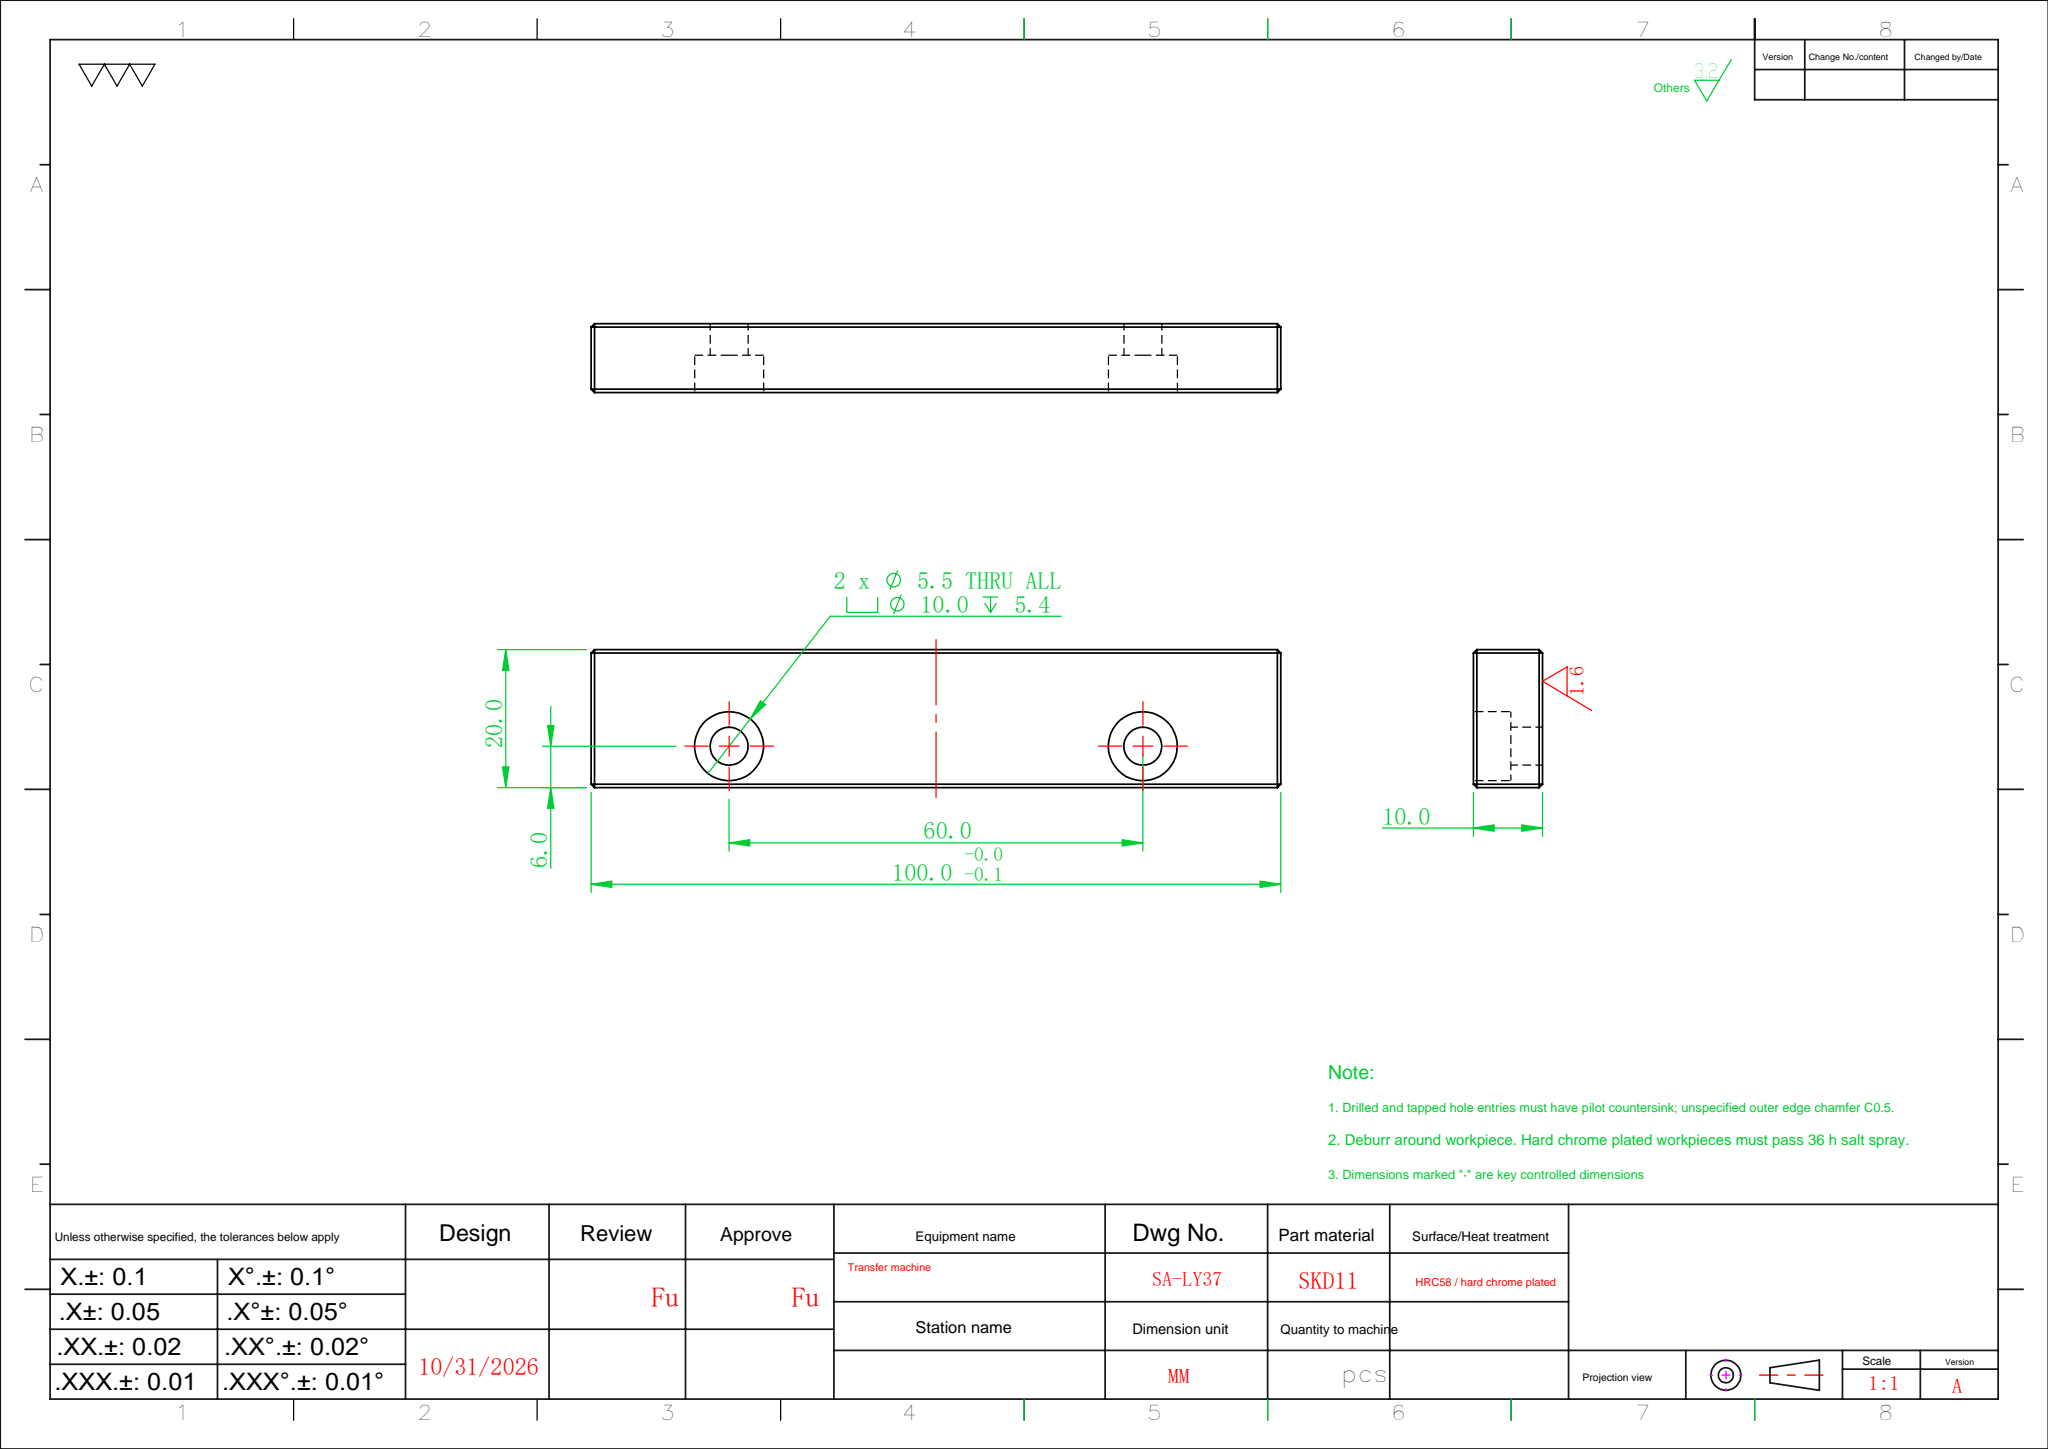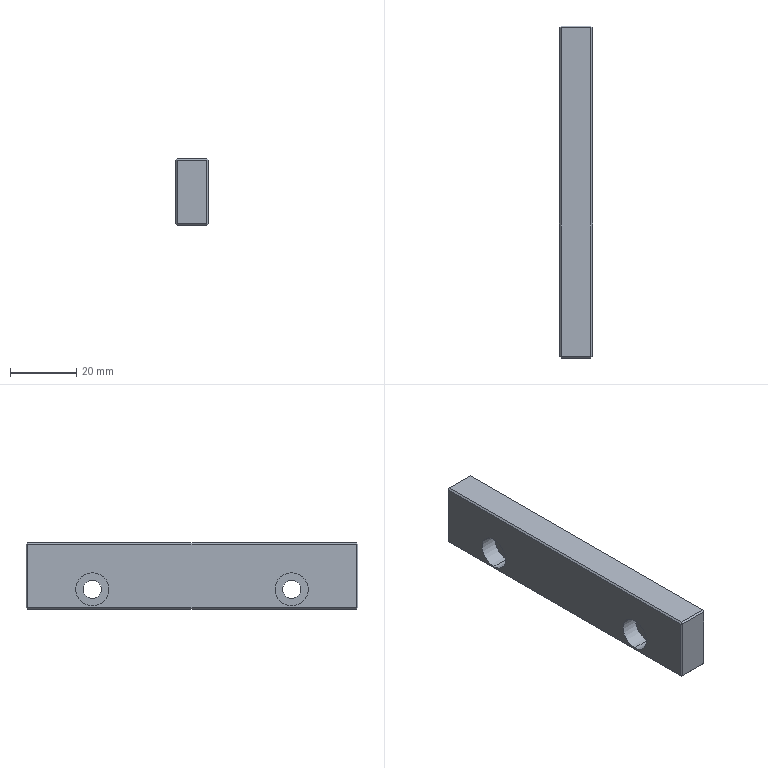Part | SolidWorks | features Chamfer 1, Extrusion 1, HoleWzd 1 | 1 solid | 36 faces | box 10 x 100 x 20 mm | volume 18869 mm3 | plane 28 | cylinder 8 | commonest cylinder face diameters 5.5 x4 10 x4
STEP:
#1=CARTESIAN_POINT('',(0.4,30.,1.));
#2=VERTEX_POINT('',#1);
#3=CARTESIAN_POINT('',(0.4,30.,11.));
#4=VERTEX_POINT('',#3);
#5=CARTESIAN_POINT('',(0.4,30.,6.));
#6=DIRECTION('',(-1.,0.,0.));
#7=DIRECTION('',(0.,0.,1.));
#8=AXIS2_PLACEMENT_3D('',#5,#6,#7);
#9=CIRCLE('',#8,5.);
#10=EDGE_CURVE('',#2,#4,#9,.T.);
#11=ORIENTED_EDGE('',*,*,#10,.F.);
#12=CARTESIAN_POINT('',(-5.,30.,1.));
#13=VERTEX_POINT('',#12);
#14=CARTESIAN_POINT('',(-5.,30.,1.));
#15=DIRECTION('',(-1.,0.,0.));
#16=VECTOR('',#15,1000.);
#17=LINE('',#14,#16);
#18=EDGE_CURVE('',#2,#13,#17,.T.);
#19=ORIENTED_EDGE('',*,*,#18,.T.);
#20=CARTESIAN_POINT('',(-5.,30.,11.));
#21=VERTEX_POINT('',#20);
#22=CARTESIAN_POINT('',(-5.,30.,6.));
#23=DIRECTION('',(-1.,0.,0.));
#24=DIRECTION('',(0.,0.,1.));
#25=AXIS2_PLACEMENT_3D('',#22,#23,#24);
#26=CIRCLE('',#25,5.);
#27=EDGE_CURVE('',#13,#21,#26,.T.);
#28=ORIENTED_EDGE('',*,*,#27,.T.);
#29=CARTESIAN_POINT('',(-5.,30.,11.));
#30=DIRECTION('',(-1.,0.,0.));
#31=VECTOR('',#30,1000.);
#32=LINE('',#29,#31);
#33=EDGE_CURVE('',#4,#21,#32,.T.);
#34=ORIENTED_EDGE('',*,*,#33,.F.);
#35=EDGE_LOOP('',(#11,#19,#28,#34));
#36=FACE_OUTER_BOUND('',#35,.T.);
#37=CARTESIAN_POINT('',(-5.,30.,6.));
#38=DIRECTION('',(-1.,0.,0.));
#39=DIRECTION('',(0.,0.,1.));
#40=AXIS2_PLACEMENT_3D('',#37,#38,#39);
#41=CYLINDRICAL_SURFACE('',#40,5.);
#42=ADVANCED_FACE('',(#36),#41,.F.);
#43=CARTESIAN_POINT('',(5.,30.,3.25));
#44=VERTEX_POINT('',#43);
#45=CARTESIAN_POINT('',(5.,30.,8.75));
#46=VERTEX_POINT('',#45);
#47=CARTESIAN_POINT('',(5.,30.,6.));
#48=DIRECTION('',(-1.,0.,0.));
#49=DIRECTION('',(0.,0.,1.));
#50=AXIS2_PLACEMENT_3D('',#47,#48,#49);
#51=CIRCLE('',#50,2.75);
#52=EDGE_CURVE('',#44,#46,#51,.T.);
#53=ORIENTED_EDGE('',*,*,#52,.F.);
#54=CARTESIAN_POINT('',(0.4,30.,3.25));
#55=VERTEX_POINT('',#54);
#56=CARTESIAN_POINT('',(-5.,30.,3.25));
#57=DIRECTION('',(-1.,0.,0.));
#58=VECTOR('',#57,1000.);
#59=LINE('',#56,#58);
#60=EDGE_CURVE('',#44,#55,#59,.T.);
#61=ORIENTED_EDGE('',*,*,#60,.T.);
#62=CARTESIAN_POINT('',(0.4,30.,8.75));
#63=VERTEX_POINT('',#62);
#64=CARTESIAN_POINT('',(0.4,30.,6.));
#65=DIRECTION('',(-1.,0.,0.));
#66=DIRECTION('',(0.,0.,1.));
#67=AXIS2_PLACEMENT_3D('',#64,#65,#66);
#68=CIRCLE('',#67,2.75);
#69=EDGE_CURVE('',#55,#63,#68,.T.);
#70=ORIENTED_EDGE('',*,*,#69,.T.);
#71=CARTESIAN_POINT('',(-5.,30.,8.75));
#72=DIRECTION('',(-1.,0.,0.));
#73=VECTOR('',#72,1000.);
#74=LINE('',#71,#73);
#75=EDGE_CURVE('',#46,#63,#74,.T.);
#76=ORIENTED_EDGE('',*,*,#75,.F.);
#77=EDGE_LOOP('',(#53,#61,#70,#76));
#78=FACE_OUTER_BOUND('',#77,.T.);
#79=CARTESIAN_POINT('',(-5.,30.,6.));
#80=DIRECTION('',(-1.,0.,0.));
#81=DIRECTION('',(0.,0.,1.));
#82=AXIS2_PLACEMENT_3D('',#79,#80,#81);
#83=CYLINDRICAL_SURFACE('',#82,2.75);
#84=ADVANCED_FACE('',(#78),#83,.F.);
#85=CARTESIAN_POINT('',(0.4,-30.,1.));
#86=VERTEX_POINT('',#85);
#87=CARTESIAN_POINT('',(0.4,-30.,11.));
#88=VERTEX_POINT('',#87);
#89=CARTESIAN_POINT('',(0.4,-30.,6.));
#90=DIRECTION('',(-1.,0.,0.));
#91=DIRECTION('',(0.,0.,1.));
#92=AXIS2_PLACEMENT_3D('',#89,#90,#91);
#93=CIRCLE('',#92,5.);
#94=EDGE_CURVE('',#86,#88,#93,.T.);
#95=ORIENTED_EDGE('',*,*,#94,.F.);
#96=CARTESIAN_POINT('',(-5.,-30.,1.));
#97=VERTEX_POINT('',#96);
#98=CARTESIAN_POINT('',(-5.,-30.,1.));
#99=DIRECTION('',(-1.,0.,0.));
#100=VECTOR('',#99,1000.);
#101=LINE('',#98,#100);
#102=EDGE_CURVE('',#86,#97,#101,.T.);
#103=ORIENTED_EDGE('',*,*,#102,.T.);
#104=CARTESIAN_POINT('',(-5.,-30.,11.));
#105=VERTEX_POINT('',#104);
#106=CARTESIAN_POINT('',(-5.,-30.,6.));
#107=DIRECTION('',(-1.,0.,0.));
#108=DIRECTION('',(0.,0.,1.));
#109=AXIS2_PLACEMENT_3D('',#106,#107,#108);
#110=CIRCLE('',#109,5.);
#111=EDGE_CURVE('',#97,#105,#110,.T.);
#112=ORIENTED_EDGE('',*,*,#111,.T.);
#113=CARTESIAN_POINT('',(-5.,-30.,11.));
#114=DIRECTION('',(-1.,0.,0.));
#115=VECTOR('',#114,1000.);
#116=LINE('',#113,#115);
#117=EDGE_CURVE('',#88,#105,#116,.T.);
#118=ORIENTED_EDGE('',*,*,#117,.F.);
#119=EDGE_LOOP('',(#95,#103,#112,#118));
#120=FACE_OUTER_BOUND('',#119,.T.);
#121=CARTESIAN_POINT('',(-5.,-30.,6.));
#122=DIRECTION('',(-1.,0.,0.));
#123=DIRECTION('',(0.,0.,1.));
#124=AXIS2_PLACEMENT_3D('',#121,#122,#123);
#125=CYLINDRICAL_SURFACE('',#124,5.);
#126=ADVANCED_FACE('',(#120),#125,.F.);
#127=CARTESIAN_POINT('',(5.,-30.,3.25));
#128=VERTEX_POINT('',#127);
#129=CARTESIAN_POINT('',(5.,-30.,8.75));
#130=VERTEX_POINT('',#129);
#131=CARTESIAN_POINT('',(5.,-30.,6.));
#132=DIRECTION('',(-1.,0.,0.));
#133=DIRECTION('',(0.,0.,1.));
#134=AXIS2_PLACEMENT_3D('',#131,#132,#133);
#135=CIRCLE('',#134,2.75);
#136=EDGE_CURVE('',#128,#130,#135,.T.);
#137=ORIENTED_EDGE('',*,*,#136,.F.);
#138=CARTESIAN_POINT('',(0.4,-30.,3.25));
#139=VERTEX_POINT('',#138);
#140=CARTESIAN_POINT('',(-5.,-30.,3.25));
#141=DIRECTION('',(-1.,0.,0.));
#142=VECTOR('',#141,1000.);
#143=LINE('',#140,#142);
#144=EDGE_CURVE('',#128,#139,#143,.T.);
#145=ORIENTED_EDGE('',*,*,#144,.T.);
#146=CARTESIAN_POINT('',(0.4,-30.,8.75));
#147=VERTEX_POINT('',#146);
#148=CARTESIAN_POINT('',(0.4,-30.,6.));
#149=DIRECTION('',(-1.,0.,0.));
#150=DIRECTION('',(0.,0.,1.));
#151=AXIS2_PLACEMENT_3D('',#148,#149,#150);
#152=CIRCLE('',#151,2.75);
#153=EDGE_CURVE('',#139,#147,#152,.T.);
#154=ORIENTED_EDGE('',*,*,#153,.T.);
#155=CARTESIAN_POINT('',(-5.,-30.,8.75));
#156=DIRECTION('',(-1.,0.,0.));
#157=VECTOR('',#156,1000.);
#158=LINE('',#155,#157);
#159=EDGE_CURVE('',#130,#147,#158,.T.);
#160=ORIENTED_EDGE('',*,*,#159,.F.);
#161=EDGE_LOOP('',(#137,#145,#154,#160));
#162=FACE_OUTER_BOUND('',#161,.T.);
#163=CARTESIAN_POINT('',(-5.,-30.,6.));
#164=DIRECTION('',(-1.,0.,0.));
#165=DIRECTION('',(0.,0.,1.));
#166=AXIS2_PLACEMENT_3D('',#163,#164,#165);
#167=CYLINDRICAL_SURFACE('',#166,2.75);
#168=ADVANCED_FACE('',(#162),#167,.F.);
#169=CARTESIAN_POINT('',(5.,49.5,19.5));
#170=VERTEX_POINT('',#169);
#171=CARTESIAN_POINT('',(5.,-49.5,19.5));
#172=VERTEX_POINT('',#171);
#173=CARTESIAN_POINT('',(5.,-50.,19.5));
#174=DIRECTION('',(0.,-1.,0.));
#175=VECTOR('',#174,1000.);
#176=LINE('',#173,#175);
#177=EDGE_CURVE('',#170,#172,#176,.T.);
#178=ORIENTED_EDGE('',*,*,#177,.T.);
#179=CARTESIAN_POINT('',(5.,-49.5,0.5));
#180=VERTEX_POINT('',#179);
#181=CARTESIAN_POINT('',(5.,-49.5,20.));
#182=DIRECTION('',(0.,0.,-1.));
#183=VECTOR('',#182,1000.);
#184=LINE('',#181,#183);
#185=EDGE_CURVE('',#172,#180,#184,.T.);
#186=ORIENTED_EDGE('',*,*,#185,.T.);
#187=CARTESIAN_POINT('',(5.,49.5,0.5));
#188=VERTEX_POINT('',#187);
#189=CARTESIAN_POINT('',(5.,50.,0.5));
#190=DIRECTION('',(0.,1.,0.));
#191=VECTOR('',#190,1000.);
#192=LINE('',#189,#191);
#193=EDGE_CURVE('',#180,#188,#192,.T.);
#194=ORIENTED_EDGE('',*,*,#193,.T.);
#195=CARTESIAN_POINT('',(5.,49.5,20.));
#196=DIRECTION('',(0.,0.,1.));
#197=VECTOR('',#196,1000.);
#198=LINE('',#195,#197);
#199=EDGE_CURVE('',#188,#170,#198,.T.);
#200=ORIENTED_EDGE('',*,*,#199,.T.);
#201=EDGE_LOOP('',(#178,#186,#194,#200));
#202=FACE_OUTER_BOUND('',#201,.T.);
#203=CARTESIAN_POINT('',(5.,30.,6.));
#204=DIRECTION('',(-1.,0.,0.));
#205=DIRECTION('',(0.,0.,1.));
#206=AXIS2_PLACEMENT_3D('',#203,#204,#205);
#207=CIRCLE('',#206,2.75);
#208=EDGE_CURVE('',#46,#44,#207,.T.);
#209=ORIENTED_EDGE('',*,*,#208,.T.);
#210=ORIENTED_EDGE('',*,*,#52,.T.);
#211=EDGE_LOOP('',(#209,#210));
#212=FACE_BOUND('',#211,.T.);
#213=CARTESIAN_POINT('',(5.,-30.,6.));
#214=DIRECTION('',(-1.,0.,0.));
#215=DIRECTION('',(0.,0.,1.));
#216=AXIS2_PLACEMENT_3D('',#213,#214,#215);
#217=CIRCLE('',#216,2.75);
#218=EDGE_CURVE('',#130,#128,#217,.T.);
#219=ORIENTED_EDGE('',*,*,#218,.T.);
#220=ORIENTED_EDGE('',*,*,#136,.T.);
#221=EDGE_LOOP('',(#219,#220));
#222=FACE_BOUND('',#221,.T.);
#223=CARTESIAN_POINT('',(5.,-50.,20.));
#224=DIRECTION('',(-1.,0.,0.));
#225=DIRECTION('',(0.,0.,1.));
#226=AXIS2_PLACEMENT_3D('',#223,#224,#225);
#227=PLANE('',#226);
#228=ADVANCED_FACE('',(#202,#212,#222),#227,.F.);
#229=CARTESIAN_POINT('',(-4.5,50.,19.5));
#230=VERTEX_POINT('',#229);
#231=CARTESIAN_POINT('',(4.5,50.,19.5));
#232=VERTEX_POINT('',#231);
#233=CARTESIAN_POINT('',(-5.,50.,19.5));
#234=DIRECTION('',(1.,0.,0.));
#235=VECTOR('',#234,1000.);
#236=LINE('',#233,#235);
#237=EDGE_CURVE('',#230,#232,#236,.T.);
#238=ORIENTED_EDGE('',*,*,#237,.T.);
#239=CARTESIAN_POINT('',(4.5,50.,0.5));
#240=VERTEX_POINT('',#239);
#241=CARTESIAN_POINT('',(4.5,50.,20.));
#242=DIRECTION('',(0.,0.,-1.));
#243=VECTOR('',#242,1000.);
#244=LINE('',#241,#243);
#245=EDGE_CURVE('',#232,#240,#244,.T.);
#246=ORIENTED_EDGE('',*,*,#245,.T.);
#247=CARTESIAN_POINT('',(-4.5,50.,0.5));
#248=VERTEX_POINT('',#247);
#249=CARTESIAN_POINT('',(-5.,50.,0.5));
#250=DIRECTION('',(-1.,0.,0.));
#251=VECTOR('',#250,1000.);
#252=LINE('',#249,#251);
#253=EDGE_CURVE('',#240,#248,#252,.T.);
#254=ORIENTED_EDGE('',*,*,#253,.T.);
#255=CARTESIAN_POINT('',(-4.5,50.,20.));
#256=DIRECTION('',(0.,0.,1.));
#257=VECTOR('',#256,1000.);
#258=LINE('',#255,#257);
#259=EDGE_CURVE('',#248,#230,#258,.T.);
#260=ORIENTED_EDGE('',*,*,#259,.T.);
#261=EDGE_LOOP('',(#238,#246,#254,#260));
#262=FACE_OUTER_BOUND('',#261,.T.);
#263=CARTESIAN_POINT('',(-5.,50.,20.));
#264=DIRECTION('',(0.,-1.,0.));
#265=DIRECTION('',(0.,0.,-1.));
#266=AXIS2_PLACEMENT_3D('',#263,#264,#265);
#267=PLANE('',#266);
#268=ADVANCED_FACE('',(#262),#267,.F.);
#269=CARTESIAN_POINT('',(-5.,-49.5,0.5));
#270=VERTEX_POINT('',#269);
#271=CARTESIAN_POINT('',(-5.,-49.5,19.5));
#272=VERTEX_POINT('',#271);
#273=CARTESIAN_POINT('',(-5.,-49.5,20.));
#274=DIRECTION('',(0.,0.,1.));
#275=VECTOR('',#274,1000.);
#276=LINE('',#273,#275);
#277=EDGE_CURVE('',#270,#272,#276,.T.);
#278=ORIENTED_EDGE('',*,*,#277,.T.);
#279=CARTESIAN_POINT('',(-5.,49.5,19.5));
#280=VERTEX_POINT('',#279);
#281=CARTESIAN_POINT('',(-5.,-50.,19.5));
#282=DIRECTION('',(0.,1.,0.));
#283=VECTOR('',#282,1000.);
#284=LINE('',#281,#283);
#285=EDGE_CURVE('',#272,#280,#284,.T.);
#286=ORIENTED_EDGE('',*,*,#285,.T.);
#287=CARTESIAN_POINT('',(-5.,49.5,0.5));
#288=VERTEX_POINT('',#287);
#289=CARTESIAN_POINT('',(-5.,49.5,20.));
#290=DIRECTION('',(0.,0.,-1.));
#291=VECTOR('',#290,1000.);
#292=LINE('',#289,#291);
#293=EDGE_CURVE('',#280,#288,#292,.T.);
#294=ORIENTED_EDGE('',*,*,#293,.T.);
#295=CARTESIAN_POINT('',(-5.,-50.,0.5));
#296=DIRECTION('',(0.,-1.,0.));
#297=VECTOR('',#296,1000.);
#298=LINE('',#295,#297);
#299=EDGE_CURVE('',#288,#270,#298,.T.);
#300=ORIENTED_EDGE('',*,*,#299,.T.);
#301=EDGE_LOOP('',(#278,#286,#294,#300));
#302=FACE_OUTER_BOUND('',#301,.T.);
#303=CARTESIAN_POINT('',(-5.,30.,6.));
#304=DIRECTION('',(-1.,0.,0.));
#305=DIRECTION('',(0.,0.,1.));
#306=AXIS2_PLACEMENT_3D('',#303,#304,#305);
#307=CIRCLE('',#306,5.);
#308=EDGE_CURVE('',#21,#13,#307,.T.);
#309=ORIENTED_EDGE('',*,*,#308,.F.);
#310=ORIENTED_EDGE('',*,*,#27,.F.);
#311=EDGE_LOOP('',(#309,#310));
#312=FACE_BOUND('',#311,.T.);
#313=CARTESIAN_POINT('',(-5.,-30.,6.));
#314=DIRECTION('',(-1.,0.,0.));
#315=DIRECTION('',(0.,0.,1.));
#316=AXIS2_PLACEMENT_3D('',#313,#314,#315);
#317=CIRCLE('',#316,5.);
#318=EDGE_CURVE('',#105,#97,#317,.T.);
#319=ORIENTED_EDGE('',*,*,#318,.F.);
#320=ORIENTED_EDGE('',*,*,#111,.F.);
#321=EDGE_LOOP('',(#319,#320));
#322=FACE_BOUND('',#321,.T.);
#323=CARTESIAN_POINT('',(-5.,-50.,20.));
#324=DIRECTION('',(1.,0.,0.));
#325=DIRECTION('',(0.,0.,-1.));
#326=AXIS2_PLACEMENT_3D('',#323,#324,#325);
#327=PLANE('',#326);
#328=ADVANCED_FACE('',(#302,#312,#322),#327,.F.);
#329=CARTESIAN_POINT('',(4.5,-50.,19.5));
#330=VERTEX_POINT('',#329);
#331=CARTESIAN_POINT('',(-4.5,-50.,19.5));
#332=VERTEX_POINT('',#331);
#333=CARTESIAN_POINT('',(-5.,-50.,19.5));
#334=DIRECTION('',(-1.,0.,0.));
#335=VECTOR('',#334,1000.);
#336=LINE('',#333,#335);
#337=EDGE_CURVE('',#330,#332,#336,.T.);
#338=ORIENTED_EDGE('',*,*,#337,.T.);
#339=CARTESIAN_POINT('',(-4.5,-50.,0.5));
#340=VERTEX_POINT('',#339);
#341=CARTESIAN_POINT('',(-4.5,-50.,20.));
#342=DIRECTION('',(0.,0.,-1.));
#343=VECTOR('',#342,1000.);
#344=LINE('',#341,#343);
#345=EDGE_CURVE('',#332,#340,#344,.T.);
#346=ORIENTED_EDGE('',*,*,#345,.T.);
#347=CARTESIAN_POINT('',(4.5,-50.,0.5));
#348=VERTEX_POINT('',#347);
#349=CARTESIAN_POINT('',(5.,-50.,0.5));
#350=DIRECTION('',(1.,0.,0.));
#351=VECTOR('',#350,1000.);
#352=LINE('',#349,#351);
#353=EDGE_CURVE('',#340,#348,#352,.T.);
#354=ORIENTED_EDGE('',*,*,#353,.T.);
#355=CARTESIAN_POINT('',(4.5,-50.,20.));
#356=DIRECTION('',(0.,0.,1.));
#357=VECTOR('',#356,1000.);
#358=LINE('',#355,#357);
#359=EDGE_CURVE('',#348,#330,#358,.T.);
#360=ORIENTED_EDGE('',*,*,#359,.T.);
#361=EDGE_LOOP('',(#338,#346,#354,#360));
#362=FACE_OUTER_BOUND('',#361,.T.);
#363=CARTESIAN_POINT('',(-5.,-50.,20.));
#364=DIRECTION('',(0.,1.,0.));
#365=DIRECTION('',(0.,0.,1.));
#366=AXIS2_PLACEMENT_3D('',#363,#364,#365);
#367=PLANE('',#366);
#368=ADVANCED_FACE('',(#362),#367,.F.);
#369=CARTESIAN_POINT('',(-4.5,49.5,20.));
#370=VERTEX_POINT('',#369);
#371=CARTESIAN_POINT('',(-4.5,-49.5,20.));
#372=VERTEX_POINT('',#371);
#373=CARTESIAN_POINT('',(-4.5,0.,20.));
#374=DIRECTION('',(0.,-1.,0.));
#375=VECTOR('',#374,1000.);
#376=LINE('',#373,#375);
#377=EDGE_CURVE('',#370,#372,#376,.T.);
#378=ORIENTED_EDGE('',*,*,#377,.T.);
#379=CARTESIAN_POINT('',(4.5,-49.5,20.));
#380=VERTEX_POINT('',#379);
#381=CARTESIAN_POINT('',(0.,-49.5,20.));
#382=DIRECTION('',(1.,0.,0.));
#383=VECTOR('',#382,1000.);
#384=LINE('',#381,#383);
#385=EDGE_CURVE('',#372,#380,#384,.T.);
#386=ORIENTED_EDGE('',*,*,#385,.T.);
#387=CARTESIAN_POINT('',(4.5,49.5,20.));
#388=VERTEX_POINT('',#387);
#389=CARTESIAN_POINT('',(4.5,0.,20.));
#390=DIRECTION('',(0.,1.,0.));
#391=VECTOR('',#390,1000.);
#392=LINE('',#389,#391);
#393=EDGE_CURVE('',#380,#388,#392,.T.);
#394=ORIENTED_EDGE('',*,*,#393,.T.);
#395=CARTESIAN_POINT('',(0.,49.5,20.));
#396=DIRECTION('',(-1.,0.,0.));
#397=VECTOR('',#396,1000.);
#398=LINE('',#395,#397);
#399=EDGE_CURVE('',#388,#370,#398,.T.);
#400=ORIENTED_EDGE('',*,*,#399,.T.);
#401=EDGE_LOOP('',(#378,#386,#394,#400));
#402=FACE_OUTER_BOUND('',#401,.T.);
#403=CARTESIAN_POINT('',(0.,0.,20.));
#404=DIRECTION('',(0.,0.,-1.));
#405=DIRECTION('',(-1.,0.,0.));
#406=AXIS2_PLACEMENT_3D('',#403,#404,#405);
#407=PLANE('',#406);
#408=ADVANCED_FACE('',(#402),#407,.F.);
#409=CARTESIAN_POINT('',(-4.5,49.5,0.));
#410=VERTEX_POINT('',#409);
#411=CARTESIAN_POINT('',(4.5,49.5,0.));
#412=VERTEX_POINT('',#411);
#413=CARTESIAN_POINT('',(5.,49.5,0.));
#414=DIRECTION('',(1.,0.,0.));
#415=VECTOR('',#414,1000.);
#416=LINE('',#413,#415);
#417=EDGE_CURVE('',#410,#412,#416,.T.);
#418=ORIENTED_EDGE('',*,*,#417,.T.);
#419=CARTESIAN_POINT('',(4.5,-49.5,0.));
#420=VERTEX_POINT('',#419);
#421=CARTESIAN_POINT('',(4.5,-50.,0.));
#422=DIRECTION('',(0.,-1.,0.));
#423=VECTOR('',#422,1000.);
#424=LINE('',#421,#423);
#425=EDGE_CURVE('',#412,#420,#424,.T.);
#426=ORIENTED_EDGE('',*,*,#425,.T.);
#427=CARTESIAN_POINT('',(-4.5,-49.5,0.));
#428=VERTEX_POINT('',#427);
#429=CARTESIAN_POINT('',(-5.,-49.5,0.));
#430=DIRECTION('',(-1.,0.,0.));
#431=VECTOR('',#430,1000.);
#432=LINE('',#429,#431);
#433=EDGE_CURVE('',#420,#428,#432,.T.);
#434=ORIENTED_EDGE('',*,*,#433,.T.);
#435=CARTESIAN_POINT('',(-4.5,50.,0.));
#436=DIRECTION('',(0.,1.,0.));
#437=VECTOR('',#436,1000.);
#438=LINE('',#435,#437);
#439=EDGE_CURVE('',#428,#410,#438,.T.);
#440=ORIENTED_EDGE('',*,*,#439,.T.);
#441=EDGE_LOOP('',(#418,#426,#434,#440));
#442=FACE_OUTER_BOUND('',#441,.T.);
#443=CARTESIAN_POINT('',(0.,0.,0.));
#444=DIRECTION('',(0.,0.,-1.));
#445=DIRECTION('',(-1.,0.,0.));
#446=AXIS2_PLACEMENT_3D('',#443,#444,#445);
#447=PLANE('',#446);
#448=ADVANCED_FACE('',(#442),#447,.T.);
#449=ORIENTED_EDGE('',*,*,#144,.F.);
#450=ORIENTED_EDGE('',*,*,#218,.F.);
#451=ORIENTED_EDGE('',*,*,#159,.T.);
#452=CARTESIAN_POINT('',(0.4,-30.,6.));
#453=DIRECTION('',(-1.,0.,0.));
#454=DIRECTION('',(0.,0.,1.));
#455=AXIS2_PLACEMENT_3D('',#452,#453,#454);
#456=CIRCLE('',#455,2.75);
#457=EDGE_CURVE('',#147,#139,#456,.T.);
#458=ORIENTED_EDGE('',*,*,#457,.T.);
#459=EDGE_LOOP('',(#449,#450,#451,#458));
#460=FACE_OUTER_BOUND('',#459,.T.);
#461=CARTESIAN_POINT('',(-5.,-30.,6.));
#462=DIRECTION('',(-1.,0.,0.));
#463=DIRECTION('',(0.,0.,1.));
#464=AXIS2_PLACEMENT_3D('',#461,#462,#463);
#465=CYLINDRICAL_SURFACE('',#464,2.75);
#466=ADVANCED_FACE('',(#460),#465,.F.);
#467=ORIENTED_EDGE('',*,*,#457,.F.);
#468=ORIENTED_EDGE('',*,*,#153,.F.);
#469=EDGE_LOOP('',(#467,#468));
#470=FACE_BOUND('',#469,.T.);
#471=CARTESIAN_POINT('',(0.4,-30.,6.));
#472=DIRECTION('',(-1.,0.,0.));
#473=DIRECTION('',(0.,0.,1.));
#474=AXIS2_PLACEMENT_3D('',#471,#472,#473);
#475=CIRCLE('',#474,5.);
#476=EDGE_CURVE('',#88,#86,#475,.T.);
#477=ORIENTED_EDGE('',*,*,#476,.T.);
#478=ORIENTED_EDGE('',*,*,#94,.T.);
#479=EDGE_LOOP('',(#477,#478));
#480=FACE_OUTER_BOUND('',#479,.T.);
#481=CARTESIAN_POINT('',(0.4,-27.25,6.));
#482=DIRECTION('',(1.,0.,0.));
#483=DIRECTION('',(0.,0.,-1.));
#484=AXIS2_PLACEMENT_3D('',#481,#482,#483);
#485=PLANE('',#484);
#486=ADVANCED_FACE('',(#470,#480),#485,.F.);
#487=ORIENTED_EDGE('',*,*,#102,.F.);
#488=ORIENTED_EDGE('',*,*,#476,.F.);
#489=ORIENTED_EDGE('',*,*,#117,.T.);
#490=ORIENTED_EDGE('',*,*,#318,.T.);
#491=EDGE_LOOP('',(#487,#488,#489,#490));
#492=FACE_OUTER_BOUND('',#491,.T.);
#493=CARTESIAN_POINT('',(-5.,-30.,6.));
#494=DIRECTION('',(-1.,0.,0.));
#495=DIRECTION('',(0.,0.,1.));
#496=AXIS2_PLACEMENT_3D('',#493,#494,#495);
#497=CYLINDRICAL_SURFACE('',#496,5.);
#498=ADVANCED_FACE('',(#492),#497,.F.);
#499=ORIENTED_EDGE('',*,*,#60,.F.);
#500=ORIENTED_EDGE('',*,*,#208,.F.);
#501=ORIENTED_EDGE('',*,*,#75,.T.);
#502=CARTESIAN_POINT('',(0.4,30.,6.));
#503=DIRECTION('',(-1.,0.,0.));
#504=DIRECTION('',(0.,0.,1.));
#505=AXIS2_PLACEMENT_3D('',#502,#503,#504);
#506=CIRCLE('',#505,2.75);
#507=EDGE_CURVE('',#63,#55,#506,.T.);
#508=ORIENTED_EDGE('',*,*,#507,.T.);
#509=EDGE_LOOP('',(#499,#500,#501,#508));
#510=FACE_OUTER_BOUND('',#509,.T.);
#511=CARTESIAN_POINT('',(-5.,30.,6.));
#512=DIRECTION('',(-1.,0.,0.));
#513=DIRECTION('',(0.,0.,1.));
#514=AXIS2_PLACEMENT_3D('',#511,#512,#513);
#515=CYLINDRICAL_SURFACE('',#514,2.75);
#516=ADVANCED_FACE('',(#510),#515,.F.);
#517=ORIENTED_EDGE('',*,*,#507,.F.);
#518=ORIENTED_EDGE('',*,*,#69,.F.);
#519=EDGE_LOOP('',(#517,#518));
#520=FACE_BOUND('',#519,.T.);
#521=CARTESIAN_POINT('',(0.4,30.,6.));
#522=DIRECTION('',(-1.,0.,0.));
#523=DIRECTION('',(0.,0.,1.));
#524=AXIS2_PLACEMENT_3D('',#521,#522,#523);
#525=CIRCLE('',#524,5.);
#526=EDGE_CURVE('',#4,#2,#525,.T.);
#527=ORIENTED_EDGE('',*,*,#526,.T.);
#528=ORIENTED_EDGE('',*,*,#10,.T.);
#529=EDGE_LOOP('',(#527,#528));
#530=FACE_OUTER_BOUND('',#529,.T.);
#531=CARTESIAN_POINT('',(0.4,32.75,6.));
#532=DIRECTION('',(1.,0.,0.));
#533=DIRECTION('',(0.,0.,-1.));
#534=AXIS2_PLACEMENT_3D('',#531,#532,#533);
#535=PLANE('',#534);
#536=ADVANCED_FACE('',(#520,#530),#535,.F.);
#537=ORIENTED_EDGE('',*,*,#18,.F.);
#538=ORIENTED_EDGE('',*,*,#526,.F.);
#539=ORIENTED_EDGE('',*,*,#33,.T.);
#540=ORIENTED_EDGE('',*,*,#308,.T.);
#541=EDGE_LOOP('',(#537,#538,#539,#540));
#542=FACE_OUTER_BOUND('',#541,.T.);
#543=CARTESIAN_POINT('',(-5.,30.,6.));
#544=DIRECTION('',(-1.,0.,0.));
#545=DIRECTION('',(0.,0.,1.));
#546=AXIS2_PLACEMENT_3D('',#543,#544,#545);
#547=CYLINDRICAL_SURFACE('',#546,5.);
#548=ADVANCED_FACE('',(#542),#547,.F.);
#549=CARTESIAN_POINT('',(-4.75,-49.5,0.25));
#550=DIRECTION('',(0.7071,0.,-0.7071));
#551=VECTOR('',#550,1000.);
#552=LINE('',#549,#551);
#553=EDGE_CURVE('',#270,#428,#552,.T.);
#554=ORIENTED_EDGE('',*,*,#553,.F.);
#555=ORIENTED_EDGE('',*,*,#299,.F.);
#556=CARTESIAN_POINT('',(-4.5,49.5,0.));
#557=DIRECTION('',(-0.7071,0.,0.7071));
#558=VECTOR('',#557,1000.);
#559=LINE('',#556,#558);
#560=EDGE_CURVE('',#410,#288,#559,.T.);
#561=ORIENTED_EDGE('',*,*,#560,.F.);
#562=ORIENTED_EDGE('',*,*,#439,.F.);
#563=EDGE_LOOP('',(#554,#555,#561,#562));
#564=FACE_OUTER_BOUND('',#563,.T.);
#565=CARTESIAN_POINT('',(-5.,-50.,0.5));
#566=DIRECTION('',(-0.7071,0.,-0.7071));
#567=DIRECTION('',(0.,1.,0.));
#568=AXIS2_PLACEMENT_3D('',#565,#566,#567);
#569=PLANE('',#568);
#570=ADVANCED_FACE('',(#564),#569,.T.);
#571=CARTESIAN_POINT('',(-4.5,-50.,0.5));
#572=DIRECTION('',(0.7071,-0.7071,0.));
#573=VECTOR('',#572,1000.);
#574=LINE('',#571,#573);
#575=EDGE_CURVE('',#270,#340,#574,.T.);
#576=ORIENTED_EDGE('',*,*,#575,.F.);
#577=ORIENTED_EDGE('',*,*,#553,.T.);
#578=CARTESIAN_POINT('',(-4.5,-50.,0.5));
#579=DIRECTION('',(0.,0.7071,-0.7071));
#580=VECTOR('',#579,1000.);
#581=LINE('',#578,#580);
#582=EDGE_CURVE('',#340,#428,#581,.T.);
#583=ORIENTED_EDGE('',*,*,#582,.F.);
#584=EDGE_LOOP('',(#576,#577,#583));
#585=FACE_OUTER_BOUND('',#584,.T.);
#586=CARTESIAN_POINT('',(-4.5,-50.,0.5));
#587=DIRECTION('',(-0.5774,-0.5774,-0.5774));
#588=DIRECTION('',(-0.7071,0.,0.7071));
#589=AXIS2_PLACEMENT_3D('',#586,#587,#588);
#590=PLANE('',#589);
#591=ADVANCED_FACE('',(#585),#590,.T.);
#592=CARTESIAN_POINT('',(-4.5,49.5,0.));
#593=DIRECTION('',(0.,0.7071,0.7071));
#594=VECTOR('',#593,1000.);
#595=LINE('',#592,#594);
#596=EDGE_CURVE('',#410,#248,#595,.T.);
#597=ORIENTED_EDGE('',*,*,#596,.F.);
#598=ORIENTED_EDGE('',*,*,#560,.T.);
#599=CARTESIAN_POINT('',(-4.75,49.75,0.5));
#600=DIRECTION('',(-0.7071,-0.7071,0.));
#601=VECTOR('',#600,1000.);
#602=LINE('',#599,#601);
#603=EDGE_CURVE('',#248,#288,#602,.T.);
#604=ORIENTED_EDGE('',*,*,#603,.F.);
#605=EDGE_LOOP('',(#597,#598,#604));
#606=FACE_OUTER_BOUND('',#605,.T.);
#607=CARTESIAN_POINT('',(-4.5,49.5,0.));
#608=DIRECTION('',(-0.5774,0.5774,-0.5774));
#609=DIRECTION('',(-0.7071,0.,0.7071));
#610=AXIS2_PLACEMENT_3D('',#607,#608,#609);
#611=PLANE('',#610);
#612=ADVANCED_FACE('',(#606),#611,.T.);
#613=ORIENTED_EDGE('',*,*,#582,.T.);
#614=ORIENTED_EDGE('',*,*,#433,.F.);
#615=CARTESIAN_POINT('',(4.5,-49.5,0.));
#616=DIRECTION('',(0.,0.7071,-0.7071));
#617=VECTOR('',#616,1000.);
#618=LINE('',#615,#617);
#619=EDGE_CURVE('',#348,#420,#618,.T.);
#620=ORIENTED_EDGE('',*,*,#619,.F.);
#621=ORIENTED_EDGE('',*,*,#353,.F.);
#622=EDGE_LOOP('',(#613,#614,#620,#621));
#623=FACE_OUTER_BOUND('',#622,.T.);
#624=CARTESIAN_POINT('',(-5.,-50.,0.5));
#625=DIRECTION('',(0.,-0.7071,-0.7071));
#626=DIRECTION('',(-1.,0.,0.));
#627=AXIS2_PLACEMENT_3D('',#624,#625,#626);
#628=PLANE('',#627);
#629=ADVANCED_FACE('',(#623),#628,.T.);
#630=ORIENTED_EDGE('',*,*,#575,.T.);
#631=ORIENTED_EDGE('',*,*,#345,.F.);
#632=CARTESIAN_POINT('',(-4.75,-49.75,19.5));
#633=DIRECTION('',(0.7071,-0.7071,0.));
#634=VECTOR('',#633,1000.);
#635=LINE('',#632,#634);
#636=EDGE_CURVE('',#272,#332,#635,.T.);
#637=ORIENTED_EDGE('',*,*,#636,.F.);
#638=ORIENTED_EDGE('',*,*,#277,.F.);
#639=EDGE_LOOP('',(#630,#631,#637,#638));
#640=FACE_OUTER_BOUND('',#639,.T.);
#641=CARTESIAN_POINT('',(-4.5,-50.,20.));
#642=DIRECTION('',(0.7071,0.7071,0.));
#643=DIRECTION('',(0.,0.,-1.));
#644=AXIS2_PLACEMENT_3D('',#641,#642,#643);
#645=PLANE('',#644);
#646=ADVANCED_FACE('',(#640),#645,.F.);
#647=CARTESIAN_POINT('',(-5.,49.5,19.5));
#648=DIRECTION('',(0.7071,0.,0.7071));
#649=VECTOR('',#648,1000.);
#650=LINE('',#647,#649);
#651=EDGE_CURVE('',#280,#370,#650,.T.);
#652=ORIENTED_EDGE('',*,*,#651,.F.);
#653=ORIENTED_EDGE('',*,*,#285,.F.);
#654=CARTESIAN_POINT('',(-4.5,-49.5,20.));
#655=DIRECTION('',(-0.7071,0.,-0.7071));
#656=VECTOR('',#655,1000.);
#657=LINE('',#654,#656);
#658=EDGE_CURVE('',#372,#272,#657,.T.);
#659=ORIENTED_EDGE('',*,*,#658,.F.);
#660=ORIENTED_EDGE('',*,*,#377,.F.);
#661=EDGE_LOOP('',(#652,#653,#659,#660));
#662=FACE_OUTER_BOUND('',#661,.T.);
#663=CARTESIAN_POINT('',(-4.5,0.,20.));
#664=DIRECTION('',(0.7071,0.,-0.7071));
#665=DIRECTION('',(0.,-1.,0.));
#666=AXIS2_PLACEMENT_3D('',#663,#664,#665);
#667=PLANE('',#666);
#668=ADVANCED_FACE('',(#662),#667,.F.);
#669=ORIENTED_EDGE('',*,*,#603,.T.);
#670=ORIENTED_EDGE('',*,*,#293,.F.);
#671=CARTESIAN_POINT('',(-5.,49.5,19.5));
#672=DIRECTION('',(-0.7071,-0.7071,0.));
#673=VECTOR('',#672,1000.);
#674=LINE('',#671,#673);
#675=EDGE_CURVE('',#230,#280,#674,.T.);
#676=ORIENTED_EDGE('',*,*,#675,.F.);
#677=ORIENTED_EDGE('',*,*,#259,.F.);
#678=EDGE_LOOP('',(#669,#670,#676,#677));
#679=FACE_OUTER_BOUND('',#678,.T.);
#680=CARTESIAN_POINT('',(-5.,49.5,20.));
#681=DIRECTION('',(0.7071,-0.7071,0.));
#682=DIRECTION('',(0.,0.,-1.));
#683=AXIS2_PLACEMENT_3D('',#680,#681,#682);
#684=PLANE('',#683);
#685=ADVANCED_FACE('',(#679),#684,.F.);
#686=ORIENTED_EDGE('',*,*,#596,.T.);
#687=ORIENTED_EDGE('',*,*,#253,.F.);
#688=CARTESIAN_POINT('',(4.5,49.75,0.25));
#689=DIRECTION('',(0.,0.7071,0.7071));
#690=VECTOR('',#689,1000.);
#691=LINE('',#688,#690);
#692=EDGE_CURVE('',#412,#240,#691,.T.);
#693=ORIENTED_EDGE('',*,*,#692,.F.);
#694=ORIENTED_EDGE('',*,*,#417,.F.);
#695=EDGE_LOOP('',(#686,#687,#693,#694));
#696=FACE_OUTER_BOUND('',#695,.T.);
#697=CARTESIAN_POINT('',(-5.,50.,0.5));
#698=DIRECTION('',(0.,0.7071,-0.7071));
#699=DIRECTION('',(1.,0.,0.));
#700=AXIS2_PLACEMENT_3D('',#697,#698,#699);
#701=PLANE('',#700);
#702=ADVANCED_FACE('',(#696),#701,.T.);
#703=CARTESIAN_POINT('',(4.5,-49.5,0.));
#704=DIRECTION('',(0.7071,0.,0.7071));
#705=VECTOR('',#704,1000.);
#706=LINE('',#703,#705);
#707=EDGE_CURVE('',#420,#180,#706,.T.);
#708=ORIENTED_EDGE('',*,*,#707,.F.);
#709=ORIENTED_EDGE('',*,*,#425,.F.);
#710=CARTESIAN_POINT('',(5.,49.5,0.5));
#711=DIRECTION('',(-0.7071,0.,-0.7071));
#712=VECTOR('',#711,1000.);
#713=LINE('',#710,#712);
#714=EDGE_CURVE('',#188,#412,#713,.T.);
#715=ORIENTED_EDGE('',*,*,#714,.F.);
#716=ORIENTED_EDGE('',*,*,#193,.F.);
#717=EDGE_LOOP('',(#708,#709,#715,#716));
#718=FACE_OUTER_BOUND('',#717,.T.);
#719=CARTESIAN_POINT('',(5.,-50.,0.5));
#720=DIRECTION('',(0.7071,0.,-0.7071));
#721=DIRECTION('',(0.,-1.,0.));
#722=AXIS2_PLACEMENT_3D('',#719,#720,#721);
#723=PLANE('',#722);
#724=ADVANCED_FACE('',(#718),#723,.T.);
#725=ORIENTED_EDGE('',*,*,#619,.T.);
#726=ORIENTED_EDGE('',*,*,#707,.T.);
#727=CARTESIAN_POINT('',(4.75,-49.75,0.5));
#728=DIRECTION('',(0.7071,0.7071,0.));
#729=VECTOR('',#728,1000.);
#730=LINE('',#727,#729);
#731=EDGE_CURVE('',#348,#180,#730,.T.);
#732=ORIENTED_EDGE('',*,*,#731,.F.);
#733=EDGE_LOOP('',(#725,#726,#732));
#734=FACE_OUTER_BOUND('',#733,.T.);
#735=CARTESIAN_POINT('',(4.5,-49.5,0.));
#736=DIRECTION('',(0.5774,-0.5774,-0.5774));
#737=DIRECTION('',(-0.7071,0.,-0.7071));
#738=AXIS2_PLACEMENT_3D('',#735,#736,#737);
#739=PLANE('',#738);
#740=ADVANCED_FACE('',(#734),#739,.T.);
#741=ORIENTED_EDGE('',*,*,#658,.T.);
#742=ORIENTED_EDGE('',*,*,#636,.T.);
#743=CARTESIAN_POINT('',(-4.5,-49.5,20.));
#744=DIRECTION('',(0.,-0.7071,-0.7071));
#745=VECTOR('',#744,1000.);
#746=LINE('',#743,#745);
#747=EDGE_CURVE('',#372,#332,#746,.T.);
#748=ORIENTED_EDGE('',*,*,#747,.F.);
#749=EDGE_LOOP('',(#741,#742,#748));
#750=FACE_OUTER_BOUND('',#749,.T.);
#751=CARTESIAN_POINT('',(-4.5,-49.5,20.));
#752=DIRECTION('',(-0.5774,-0.5774,0.5774));
#753=DIRECTION('',(0.7071,0.,0.7071));
#754=AXIS2_PLACEMENT_3D('',#751,#752,#753);
#755=PLANE('',#754);
#756=ADVANCED_FACE('',(#750),#755,.T.);
#757=ORIENTED_EDGE('',*,*,#675,.T.);
#758=ORIENTED_EDGE('',*,*,#651,.T.);
#759=CARTESIAN_POINT('',(-4.5,49.75,19.75));
#760=DIRECTION('',(0.,-0.7071,0.7071));
#761=VECTOR('',#760,1000.);
#762=LINE('',#759,#761);
#763=EDGE_CURVE('',#230,#370,#762,.T.);
#764=ORIENTED_EDGE('',*,*,#763,.F.);
#765=EDGE_LOOP('',(#757,#758,#764));
#766=FACE_OUTER_BOUND('',#765,.T.);
#767=CARTESIAN_POINT('',(-5.,49.5,19.5));
#768=DIRECTION('',(-0.5774,0.5774,0.5774));
#769=DIRECTION('',(0.7071,0.,0.7071));
#770=AXIS2_PLACEMENT_3D('',#767,#768,#769);
#771=PLANE('',#770);
#772=ADVANCED_FACE('',(#766),#771,.T.);
#773=ORIENTED_EDGE('',*,*,#714,.T.);
#774=ORIENTED_EDGE('',*,*,#692,.T.);
#775=CARTESIAN_POINT('',(5.,49.5,0.5));
#776=DIRECTION('',(-0.7071,0.7071,0.));
#777=VECTOR('',#776,1000.);
#778=LINE('',#775,#777);
#779=EDGE_CURVE('',#188,#240,#778,.T.);
#780=ORIENTED_EDGE('',*,*,#779,.F.);
#781=EDGE_LOOP('',(#773,#774,#780));
#782=FACE_OUTER_BOUND('',#781,.T.);
#783=CARTESIAN_POINT('',(5.,49.5,0.5));
#784=DIRECTION('',(0.5774,0.5774,-0.5774));
#785=DIRECTION('',(-0.7071,0.,-0.7071));
#786=AXIS2_PLACEMENT_3D('',#783,#784,#785);
#787=PLANE('',#786);
#788=ADVANCED_FACE('',(#782),#787,.T.);
#789=ORIENTED_EDGE('',*,*,#731,.T.);
#790=ORIENTED_EDGE('',*,*,#185,.F.);
#791=CARTESIAN_POINT('',(5.,-49.5,19.5));
#792=DIRECTION('',(0.7071,0.7071,0.));
#793=VECTOR('',#792,1000.);
#794=LINE('',#791,#793);
#795=EDGE_CURVE('',#330,#172,#794,.T.);
#796=ORIENTED_EDGE('',*,*,#795,.F.);
#797=ORIENTED_EDGE('',*,*,#359,.F.);
#798=EDGE_LOOP('',(#789,#790,#796,#797));
#799=FACE_OUTER_BOUND('',#798,.T.);
#800=CARTESIAN_POINT('',(5.,-49.5,20.));
#801=DIRECTION('',(-0.7071,0.7071,0.));
#802=DIRECTION('',(0.,0.,-1.));
#803=AXIS2_PLACEMENT_3D('',#800,#801,#802);
#804=PLANE('',#803);
#805=ADVANCED_FACE('',(#799),#804,.F.);
#806=ORIENTED_EDGE('',*,*,#747,.T.);
#807=ORIENTED_EDGE('',*,*,#337,.F.);
#808=CARTESIAN_POINT('',(4.5,-49.75,19.75));
#809=DIRECTION('',(0.,-0.7071,-0.7071));
#810=VECTOR('',#809,1000.);
#811=LINE('',#808,#810);
#812=EDGE_CURVE('',#380,#330,#811,.T.);
#813=ORIENTED_EDGE('',*,*,#812,.F.);
#814=ORIENTED_EDGE('',*,*,#385,.F.);
#815=EDGE_LOOP('',(#806,#807,#813,#814));
#816=FACE_OUTER_BOUND('',#815,.T.);
#817=CARTESIAN_POINT('',(0.,-49.5,20.));
#818=DIRECTION('',(0.,0.7071,-0.7071));
#819=DIRECTION('',(1.,0.,0.));
#820=AXIS2_PLACEMENT_3D('',#817,#818,#819);
#821=PLANE('',#820);
#822=ADVANCED_FACE('',(#816),#821,.F.);
#823=ORIENTED_EDGE('',*,*,#763,.T.);
#824=ORIENTED_EDGE('',*,*,#399,.F.);
#825=CARTESIAN_POINT('',(4.5,49.5,20.));
#826=DIRECTION('',(0.,-0.7071,0.7071));
#827=VECTOR('',#826,1000.);
#828=LINE('',#825,#827);
#829=EDGE_CURVE('',#232,#388,#828,.T.);
#830=ORIENTED_EDGE('',*,*,#829,.F.);
#831=ORIENTED_EDGE('',*,*,#237,.F.);
#832=EDGE_LOOP('',(#823,#824,#830,#831));
#833=FACE_OUTER_BOUND('',#832,.T.);
#834=CARTESIAN_POINT('',(0.,49.5,20.));
#835=DIRECTION('',(0.,-0.7071,-0.7071));
#836=DIRECTION('',(-1.,0.,0.));
#837=AXIS2_PLACEMENT_3D('',#834,#835,#836);
#838=PLANE('',#837);
#839=ADVANCED_FACE('',(#833),#838,.F.);
#840=ORIENTED_EDGE('',*,*,#779,.T.);
#841=ORIENTED_EDGE('',*,*,#245,.F.);
#842=CARTESIAN_POINT('',(4.75,49.75,19.5));
#843=DIRECTION('',(-0.7071,0.7071,0.));
#844=VECTOR('',#843,1000.);
#845=LINE('',#842,#844);
#846=EDGE_CURVE('',#170,#232,#845,.T.);
#847=ORIENTED_EDGE('',*,*,#846,.F.);
#848=ORIENTED_EDGE('',*,*,#199,.F.);
#849=EDGE_LOOP('',(#840,#841,#847,#848));
#850=FACE_OUTER_BOUND('',#849,.T.);
#851=CARTESIAN_POINT('',(4.5,50.,20.));
#852=DIRECTION('',(-0.7071,-0.7071,0.));
#853=DIRECTION('',(0.,0.,-1.));
#854=AXIS2_PLACEMENT_3D('',#851,#852,#853);
#855=PLANE('',#854);
#856=ADVANCED_FACE('',(#850),#855,.F.);
#857=ORIENTED_EDGE('',*,*,#812,.T.);
#858=ORIENTED_EDGE('',*,*,#795,.T.);
#859=CARTESIAN_POINT('',(5.,-49.5,19.5));
#860=DIRECTION('',(0.7071,0.,-0.7071));
#861=VECTOR('',#860,1000.);
#862=LINE('',#859,#861);
#863=EDGE_CURVE('',#380,#172,#862,.T.);
#864=ORIENTED_EDGE('',*,*,#863,.F.);
#865=EDGE_LOOP('',(#857,#858,#864));
#866=FACE_OUTER_BOUND('',#865,.T.);
#867=CARTESIAN_POINT('',(5.,-49.5,19.5));
#868=DIRECTION('',(0.5774,-0.5774,0.5774));
#869=DIRECTION('',(0.7071,0.,-0.7071));
#870=AXIS2_PLACEMENT_3D('',#867,#868,#869);
#871=PLANE('',#870);
#872=ADVANCED_FACE('',(#866),#871,.T.);
#873=ORIENTED_EDGE('',*,*,#846,.T.);
#874=ORIENTED_EDGE('',*,*,#829,.T.);
#875=CARTESIAN_POINT('',(4.5,49.5,20.));
#876=DIRECTION('',(-0.7071,0.,0.7071));
#877=VECTOR('',#876,1000.);
#878=LINE('',#875,#877);
#879=EDGE_CURVE('',#170,#388,#878,.T.);
#880=ORIENTED_EDGE('',*,*,#879,.F.);
#881=EDGE_LOOP('',(#873,#874,#880));
#882=FACE_OUTER_BOUND('',#881,.T.);
#883=CARTESIAN_POINT('',(4.5,49.5,20.));
#884=DIRECTION('',(0.5774,0.5774,0.5774));
#885=DIRECTION('',(0.7071,0.,-0.7071));
#886=AXIS2_PLACEMENT_3D('',#883,#884,#885);
#887=PLANE('',#886);
#888=ADVANCED_FACE('',(#882),#887,.T.);
#889=ORIENTED_EDGE('',*,*,#863,.T.);
#890=ORIENTED_EDGE('',*,*,#177,.F.);
#891=ORIENTED_EDGE('',*,*,#879,.T.);
#892=ORIENTED_EDGE('',*,*,#393,.F.);
#893=EDGE_LOOP('',(#889,#890,#891,#892));
#894=FACE_OUTER_BOUND('',#893,.T.);
#895=CARTESIAN_POINT('',(4.5,0.,20.));
#896=DIRECTION('',(-0.7071,0.,-0.7071));
#897=DIRECTION('',(0.,1.,0.));
#898=AXIS2_PLACEMENT_3D('',#895,#896,#897);
#899=PLANE('',#898);
#900=ADVANCED_FACE('',(#894),#899,.F.);
#901=CLOSED_SHELL('',(#42,#84,#126,#168,#228,#268,#328,#368,#408,#448,#466,#486,#498,#516,#536,#548,#570,#591,#612,#629,#646,#668,#685,#702,#724,#740,#756,#772,#788,#805,#822,#839,#856,#872,#888,#900));
#902=MANIFOLD_SOLID_BREP('',#901);
#903=CARTESIAN_POINT('',(0.,0.,0.));
#904=DIRECTION('',(0.,0.,1.));
#905=DIRECTION('',(1.,0.,0.));
#906=AXIS2_PLACEMENT_3D('',#903,#904,#905);
#907=(LENGTH_UNIT()NAMED_UNIT(*)SI_UNIT(.MILLI.,.METRE.));
#908=UNCERTAINTY_MEASURE_WITH_UNIT(LENGTH_MEASURE(0.00001),#907,'','');
#909=(NAMED_UNIT(*)PLANE_ANGLE_UNIT()SI_UNIT($,.RADIAN.));
#910=(NAMED_UNIT(*)SI_UNIT($,.STERADIAN.)SOLID_ANGLE_UNIT());
#911=(GEOMETRIC_REPRESENTATION_CONTEXT(3)GLOBAL_UNCERTAINTY_ASSIGNED_CONTEXT((#908))GLOBAL_UNIT_ASSIGNED_CONTEXT((#907,#909,#910))REPRESENTATION_CONTEXT('',''));
#912=ADVANCED_BREP_SHAPE_REPRESENTATION('',(#902,#906),#911);